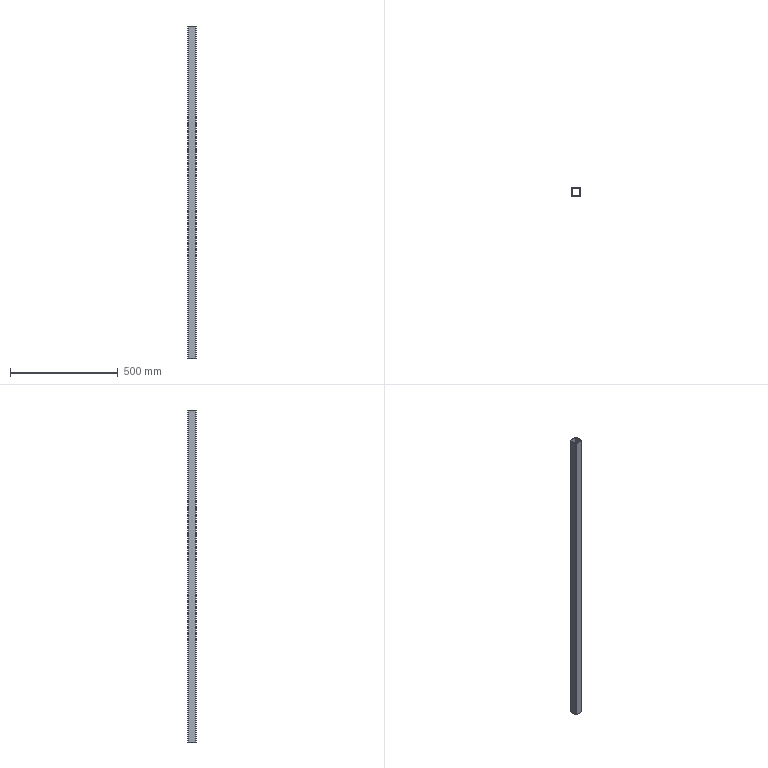Part | STEP file | X77-03115 | 1 solid | 14 faces | box 40 x 40 x 1540 mm | volume 671862 mm3 | plane 10 | cylinder 4 | commonest cylinder face diameters 6 x4
STEP:
#1=CARTESIAN_POINT('',(-20.,-17.,1540.));
#2=VERTEX_POINT('',#1);
#3=CARTESIAN_POINT('',(-17.,-20.,1540.));
#4=VERTEX_POINT('',#3);
#5=CARTESIAN_POINT('',(-17.,-17.,1540.));
#6=DIRECTION('',(0.,0.,1.));
#7=DIRECTION('',(-1.,0.,0.));
#8=AXIS2_PLACEMENT_3D('',#5,#6,#7);
#9=CIRCLE('',#8,3.);
#10=EDGE_CURVE('',#2,#4,#9,.T.);
#11=ORIENTED_EDGE('',*,*,#10,.T.);
#12=CARTESIAN_POINT('',(17.,-20.,1540.));
#13=VERTEX_POINT('',#12);
#14=CARTESIAN_POINT('',(-17.,-20.,1540.));
#15=DIRECTION('',(1.,0.,0.));
#16=VECTOR('',#15,1000.);
#17=LINE('',#14,#16);
#18=EDGE_CURVE('',#4,#13,#17,.T.);
#19=ORIENTED_EDGE('',*,*,#18,.T.);
#20=CARTESIAN_POINT('',(20.,-17.,1540.));
#21=VERTEX_POINT('',#20);
#22=CARTESIAN_POINT('',(17.,-17.,1540.));
#23=DIRECTION('',(0.,0.,1.));
#24=DIRECTION('',(-1.,0.,0.));
#25=AXIS2_PLACEMENT_3D('',#22,#23,#24);
#26=CIRCLE('',#25,3.);
#27=EDGE_CURVE('',#13,#21,#26,.T.);
#28=ORIENTED_EDGE('',*,*,#27,.T.);
#29=CARTESIAN_POINT('',(20.,17.,1540.));
#30=VERTEX_POINT('',#29);
#31=CARTESIAN_POINT('',(20.,-17.,1540.));
#32=DIRECTION('',(0.,1.,0.));
#33=VECTOR('',#32,1000.);
#34=LINE('',#31,#33);
#35=EDGE_CURVE('',#21,#30,#34,.T.);
#36=ORIENTED_EDGE('',*,*,#35,.T.);
#37=CARTESIAN_POINT('',(17.,20.,1540.));
#38=VERTEX_POINT('',#37);
#39=CARTESIAN_POINT('',(17.,17.,1540.));
#40=DIRECTION('',(0.,0.,1.));
#41=DIRECTION('',(1.,0.,0.));
#42=AXIS2_PLACEMENT_3D('',#39,#40,#41);
#43=CIRCLE('',#42,3.);
#44=EDGE_CURVE('',#30,#38,#43,.T.);
#45=ORIENTED_EDGE('',*,*,#44,.T.);
#46=CARTESIAN_POINT('',(-17.,20.,1540.));
#47=VERTEX_POINT('',#46);
#48=CARTESIAN_POINT('',(-17.,20.,1540.));
#49=DIRECTION('',(-1.,0.,0.));
#50=VECTOR('',#49,1000.);
#51=LINE('',#48,#50);
#52=EDGE_CURVE('',#38,#47,#51,.T.);
#53=ORIENTED_EDGE('',*,*,#52,.T.);
#54=CARTESIAN_POINT('',(-20.,17.,1540.));
#55=VERTEX_POINT('',#54);
#56=CARTESIAN_POINT('',(-17.,17.,1540.));
#57=DIRECTION('',(0.,0.,1.));
#58=DIRECTION('',(1.,0.,0.));
#59=AXIS2_PLACEMENT_3D('',#56,#57,#58);
#60=CIRCLE('',#59,3.);
#61=EDGE_CURVE('',#47,#55,#60,.T.);
#62=ORIENTED_EDGE('',*,*,#61,.T.);
#63=CARTESIAN_POINT('',(-20.,-17.,1540.));
#64=DIRECTION('',(0.,-1.,0.));
#65=VECTOR('',#64,1000.);
#66=LINE('',#63,#65);
#67=EDGE_CURVE('',#55,#2,#66,.T.);
#68=ORIENTED_EDGE('',*,*,#67,.T.);
#69=EDGE_LOOP('',(#11,#19,#28,#36,#45,#53,#62,#68));
#70=FACE_OUTER_BOUND('',#69,.T.);
#71=CARTESIAN_POINT('',(17.,-17.,1540.));
#72=VERTEX_POINT('',#71);
#73=CARTESIAN_POINT('',(17.,17.,1540.));
#74=VERTEX_POINT('',#73);
#75=CARTESIAN_POINT('',(17.,-17.,1540.));
#76=DIRECTION('',(0.,1.,0.));
#77=VECTOR('',#76,1000.);
#78=LINE('',#75,#77);
#79=EDGE_CURVE('',#72,#74,#78,.T.);
#80=ORIENTED_EDGE('',*,*,#79,.F.);
#81=CARTESIAN_POINT('',(-17.,-17.,1540.));
#82=VERTEX_POINT('',#81);
#83=CARTESIAN_POINT('',(-17.,-17.,1540.));
#84=DIRECTION('',(1.,0.,0.));
#85=VECTOR('',#84,1000.);
#86=LINE('',#83,#85);
#87=EDGE_CURVE('',#82,#72,#86,.T.);
#88=ORIENTED_EDGE('',*,*,#87,.F.);
#89=CARTESIAN_POINT('',(-17.,17.,1540.));
#90=VERTEX_POINT('',#89);
#91=CARTESIAN_POINT('',(-17.,-17.,1540.));
#92=DIRECTION('',(0.,-1.,0.));
#93=VECTOR('',#92,1000.);
#94=LINE('',#91,#93);
#95=EDGE_CURVE('',#90,#82,#94,.T.);
#96=ORIENTED_EDGE('',*,*,#95,.F.);
#97=CARTESIAN_POINT('',(-17.,17.,1540.));
#98=DIRECTION('',(-1.,0.,0.));
#99=VECTOR('',#98,1000.);
#100=LINE('',#97,#99);
#101=EDGE_CURVE('',#74,#90,#100,.T.);
#102=ORIENTED_EDGE('',*,*,#101,.F.);
#103=EDGE_LOOP('',(#80,#88,#96,#102));
#104=FACE_BOUND('',#103,.T.);
#105=CARTESIAN_POINT('',(-17.,-17.,1540.));
#106=DIRECTION('',(0.,0.,-1.));
#107=DIRECTION('',(-1.,0.,0.));
#108=AXIS2_PLACEMENT_3D('',#105,#106,#107);
#109=PLANE('',#108);
#110=ADVANCED_FACE('',(#70,#104),#109,.F.);
#111=CARTESIAN_POINT('',(-20.,-17.,0.));
#112=VERTEX_POINT('',#111);
#113=CARTESIAN_POINT('',(-17.,-20.,0.));
#114=VERTEX_POINT('',#113);
#115=CARTESIAN_POINT('',(-17.,-17.,0.));
#116=DIRECTION('',(0.,0.,1.));
#117=DIRECTION('',(-1.,0.,0.));
#118=AXIS2_PLACEMENT_3D('',#115,#116,#117);
#119=CIRCLE('',#118,3.);
#120=EDGE_CURVE('',#112,#114,#119,.T.);
#121=ORIENTED_EDGE('',*,*,#120,.F.);
#122=CARTESIAN_POINT('',(-20.,17.,0.));
#123=VERTEX_POINT('',#122);
#124=CARTESIAN_POINT('',(-20.,-17.,0.));
#125=DIRECTION('',(0.,-1.,0.));
#126=VECTOR('',#125,1000.);
#127=LINE('',#124,#126);
#128=EDGE_CURVE('',#123,#112,#127,.T.);
#129=ORIENTED_EDGE('',*,*,#128,.F.);
#130=CARTESIAN_POINT('',(-17.,20.,0.));
#131=VERTEX_POINT('',#130);
#132=CARTESIAN_POINT('',(-17.,17.,0.));
#133=DIRECTION('',(0.,0.,1.));
#134=DIRECTION('',(1.,0.,0.));
#135=AXIS2_PLACEMENT_3D('',#132,#133,#134);
#136=CIRCLE('',#135,3.);
#137=EDGE_CURVE('',#131,#123,#136,.T.);
#138=ORIENTED_EDGE('',*,*,#137,.F.);
#139=CARTESIAN_POINT('',(17.,20.,0.));
#140=VERTEX_POINT('',#139);
#141=CARTESIAN_POINT('',(-17.,20.,0.));
#142=DIRECTION('',(-1.,0.,0.));
#143=VECTOR('',#142,1000.);
#144=LINE('',#141,#143);
#145=EDGE_CURVE('',#140,#131,#144,.T.);
#146=ORIENTED_EDGE('',*,*,#145,.F.);
#147=CARTESIAN_POINT('',(20.,17.,0.));
#148=VERTEX_POINT('',#147);
#149=CARTESIAN_POINT('',(17.,17.,0.));
#150=DIRECTION('',(0.,0.,1.));
#151=DIRECTION('',(1.,0.,0.));
#152=AXIS2_PLACEMENT_3D('',#149,#150,#151);
#153=CIRCLE('',#152,3.);
#154=EDGE_CURVE('',#148,#140,#153,.T.);
#155=ORIENTED_EDGE('',*,*,#154,.F.);
#156=CARTESIAN_POINT('',(20.,-17.,0.));
#157=VERTEX_POINT('',#156);
#158=CARTESIAN_POINT('',(20.,-17.,0.));
#159=DIRECTION('',(0.,1.,0.));
#160=VECTOR('',#159,1000.);
#161=LINE('',#158,#160);
#162=EDGE_CURVE('',#157,#148,#161,.T.);
#163=ORIENTED_EDGE('',*,*,#162,.F.);
#164=CARTESIAN_POINT('',(17.,-20.,0.));
#165=VERTEX_POINT('',#164);
#166=CARTESIAN_POINT('',(17.,-17.,0.));
#167=DIRECTION('',(0.,0.,1.));
#168=DIRECTION('',(-1.,0.,0.));
#169=AXIS2_PLACEMENT_3D('',#166,#167,#168);
#170=CIRCLE('',#169,3.);
#171=EDGE_CURVE('',#165,#157,#170,.T.);
#172=ORIENTED_EDGE('',*,*,#171,.F.);
#173=CARTESIAN_POINT('',(-17.,-20.,0.));
#174=DIRECTION('',(1.,0.,0.));
#175=VECTOR('',#174,1000.);
#176=LINE('',#173,#175);
#177=EDGE_CURVE('',#114,#165,#176,.T.);
#178=ORIENTED_EDGE('',*,*,#177,.F.);
#179=EDGE_LOOP('',(#121,#129,#138,#146,#155,#163,#172,#178));
#180=FACE_OUTER_BOUND('',#179,.T.);
#181=CARTESIAN_POINT('',(-17.,-17.,0.));
#182=VERTEX_POINT('',#181);
#183=CARTESIAN_POINT('',(17.,-17.,0.));
#184=VERTEX_POINT('',#183);
#185=CARTESIAN_POINT('',(-17.,-17.,0.));
#186=DIRECTION('',(1.,0.,0.));
#187=VECTOR('',#186,1000.);
#188=LINE('',#185,#187);
#189=EDGE_CURVE('',#182,#184,#188,.T.);
#190=ORIENTED_EDGE('',*,*,#189,.T.);
#191=CARTESIAN_POINT('',(17.,17.,0.));
#192=VERTEX_POINT('',#191);
#193=CARTESIAN_POINT('',(17.,-17.,0.));
#194=DIRECTION('',(0.,1.,0.));
#195=VECTOR('',#194,1000.);
#196=LINE('',#193,#195);
#197=EDGE_CURVE('',#184,#192,#196,.T.);
#198=ORIENTED_EDGE('',*,*,#197,.T.);
#199=CARTESIAN_POINT('',(-17.,17.,0.));
#200=VERTEX_POINT('',#199);
#201=CARTESIAN_POINT('',(-17.,17.,0.));
#202=DIRECTION('',(-1.,0.,0.));
#203=VECTOR('',#202,1000.);
#204=LINE('',#201,#203);
#205=EDGE_CURVE('',#192,#200,#204,.T.);
#206=ORIENTED_EDGE('',*,*,#205,.T.);
#207=CARTESIAN_POINT('',(-17.,-17.,0.));
#208=DIRECTION('',(0.,-1.,0.));
#209=VECTOR('',#208,1000.);
#210=LINE('',#207,#209);
#211=EDGE_CURVE('',#200,#182,#210,.T.);
#212=ORIENTED_EDGE('',*,*,#211,.T.);
#213=EDGE_LOOP('',(#190,#198,#206,#212));
#214=FACE_BOUND('',#213,.T.);
#215=CARTESIAN_POINT('',(-17.,-17.,0.));
#216=DIRECTION('',(0.,0.,-1.));
#217=DIRECTION('',(-1.,0.,0.));
#218=AXIS2_PLACEMENT_3D('',#215,#216,#217);
#219=PLANE('',#218);
#220=ADVANCED_FACE('',(#180,#214),#219,.T.);
#221=ORIENTED_EDGE('',*,*,#120,.T.);
#222=CARTESIAN_POINT('',(-17.,-20.,1540.));
#223=DIRECTION('',(0.,0.,-1.));
#224=VECTOR('',#223,1000.);
#225=LINE('',#222,#224);
#226=EDGE_CURVE('',#4,#114,#225,.T.);
#227=ORIENTED_EDGE('',*,*,#226,.F.);
#228=ORIENTED_EDGE('',*,*,#10,.F.);
#229=CARTESIAN_POINT('',(-20.,-17.,1540.));
#230=DIRECTION('',(0.,0.,-1.));
#231=VECTOR('',#230,1000.);
#232=LINE('',#229,#231);
#233=EDGE_CURVE('',#2,#112,#232,.T.);
#234=ORIENTED_EDGE('',*,*,#233,.T.);
#235=EDGE_LOOP('',(#221,#227,#228,#234));
#236=FACE_OUTER_BOUND('',#235,.T.);
#237=CARTESIAN_POINT('',(-17.,-17.,1540.));
#238=DIRECTION('',(0.,0.,-1.));
#239=DIRECTION('',(-1.,0.,0.));
#240=AXIS2_PLACEMENT_3D('',#237,#238,#239);
#241=CYLINDRICAL_SURFACE('',#240,3.);
#242=ADVANCED_FACE('',(#236),#241,.T.);
#243=ORIENTED_EDGE('',*,*,#177,.T.);
#244=CARTESIAN_POINT('',(17.,-20.,1540.));
#245=DIRECTION('',(0.,0.,-1.));
#246=VECTOR('',#245,1000.);
#247=LINE('',#244,#246);
#248=EDGE_CURVE('',#13,#165,#247,.T.);
#249=ORIENTED_EDGE('',*,*,#248,.F.);
#250=ORIENTED_EDGE('',*,*,#18,.F.);
#251=ORIENTED_EDGE('',*,*,#226,.T.);
#252=EDGE_LOOP('',(#243,#249,#250,#251));
#253=FACE_OUTER_BOUND('',#252,.T.);
#254=CARTESIAN_POINT('',(-17.,-20.,1540.));
#255=DIRECTION('',(0.,1.,0.));
#256=DIRECTION('',(0.,0.,1.));
#257=AXIS2_PLACEMENT_3D('',#254,#255,#256);
#258=PLANE('',#257);
#259=ADVANCED_FACE('',(#253),#258,.F.);
#260=ORIENTED_EDGE('',*,*,#171,.T.);
#261=CARTESIAN_POINT('',(20.,-17.,1540.));
#262=DIRECTION('',(0.,0.,-1.));
#263=VECTOR('',#262,1000.);
#264=LINE('',#261,#263);
#265=EDGE_CURVE('',#21,#157,#264,.T.);
#266=ORIENTED_EDGE('',*,*,#265,.F.);
#267=ORIENTED_EDGE('',*,*,#27,.F.);
#268=ORIENTED_EDGE('',*,*,#248,.T.);
#269=EDGE_LOOP('',(#260,#266,#267,#268));
#270=FACE_OUTER_BOUND('',#269,.T.);
#271=CARTESIAN_POINT('',(17.,-17.,1540.));
#272=DIRECTION('',(0.,0.,-1.));
#273=DIRECTION('',(-1.,0.,0.));
#274=AXIS2_PLACEMENT_3D('',#271,#272,#273);
#275=CYLINDRICAL_SURFACE('',#274,3.);
#276=ADVANCED_FACE('',(#270),#275,.T.);
#277=ORIENTED_EDGE('',*,*,#162,.T.);
#278=CARTESIAN_POINT('',(20.,17.,1540.));
#279=DIRECTION('',(0.,0.,-1.));
#280=VECTOR('',#279,1000.);
#281=LINE('',#278,#280);
#282=EDGE_CURVE('',#30,#148,#281,.T.);
#283=ORIENTED_EDGE('',*,*,#282,.F.);
#284=ORIENTED_EDGE('',*,*,#35,.F.);
#285=ORIENTED_EDGE('',*,*,#265,.T.);
#286=EDGE_LOOP('',(#277,#283,#284,#285));
#287=FACE_OUTER_BOUND('',#286,.T.);
#288=CARTESIAN_POINT('',(20.,-17.,1540.));
#289=DIRECTION('',(-1.,0.,0.));
#290=DIRECTION('',(0.,0.,1.));
#291=AXIS2_PLACEMENT_3D('',#288,#289,#290);
#292=PLANE('',#291);
#293=ADVANCED_FACE('',(#287),#292,.F.);
#294=ORIENTED_EDGE('',*,*,#154,.T.);
#295=CARTESIAN_POINT('',(17.,20.,1540.));
#296=DIRECTION('',(0.,0.,-1.));
#297=VECTOR('',#296,1000.);
#298=LINE('',#295,#297);
#299=EDGE_CURVE('',#38,#140,#298,.T.);
#300=ORIENTED_EDGE('',*,*,#299,.F.);
#301=ORIENTED_EDGE('',*,*,#44,.F.);
#302=ORIENTED_EDGE('',*,*,#282,.T.);
#303=EDGE_LOOP('',(#294,#300,#301,#302));
#304=FACE_OUTER_BOUND('',#303,.T.);
#305=CARTESIAN_POINT('',(17.,17.,1540.));
#306=DIRECTION('',(0.,0.,-1.));
#307=DIRECTION('',(-1.,0.,0.));
#308=AXIS2_PLACEMENT_3D('',#305,#306,#307);
#309=CYLINDRICAL_SURFACE('',#308,3.);
#310=ADVANCED_FACE('',(#304),#309,.T.);
#311=ORIENTED_EDGE('',*,*,#145,.T.);
#312=CARTESIAN_POINT('',(-17.,20.,1540.));
#313=DIRECTION('',(0.,0.,-1.));
#314=VECTOR('',#313,1000.);
#315=LINE('',#312,#314);
#316=EDGE_CURVE('',#47,#131,#315,.T.);
#317=ORIENTED_EDGE('',*,*,#316,.F.);
#318=ORIENTED_EDGE('',*,*,#52,.F.);
#319=ORIENTED_EDGE('',*,*,#299,.T.);
#320=EDGE_LOOP('',(#311,#317,#318,#319));
#321=FACE_OUTER_BOUND('',#320,.T.);
#322=CARTESIAN_POINT('',(-17.,20.,1540.));
#323=DIRECTION('',(0.,-1.,0.));
#324=DIRECTION('',(0.,0.,-1.));
#325=AXIS2_PLACEMENT_3D('',#322,#323,#324);
#326=PLANE('',#325);
#327=ADVANCED_FACE('',(#321),#326,.F.);
#328=ORIENTED_EDGE('',*,*,#137,.T.);
#329=CARTESIAN_POINT('',(-20.,17.,1540.));
#330=DIRECTION('',(0.,0.,-1.));
#331=VECTOR('',#330,1000.);
#332=LINE('',#329,#331);
#333=EDGE_CURVE('',#55,#123,#332,.T.);
#334=ORIENTED_EDGE('',*,*,#333,.F.);
#335=ORIENTED_EDGE('',*,*,#61,.F.);
#336=ORIENTED_EDGE('',*,*,#316,.T.);
#337=EDGE_LOOP('',(#328,#334,#335,#336));
#338=FACE_OUTER_BOUND('',#337,.T.);
#339=CARTESIAN_POINT('',(-17.,17.,1540.));
#340=DIRECTION('',(0.,0.,-1.));
#341=DIRECTION('',(-1.,0.,0.));
#342=AXIS2_PLACEMENT_3D('',#339,#340,#341);
#343=CYLINDRICAL_SURFACE('',#342,3.);
#344=ADVANCED_FACE('',(#338),#343,.T.);
#345=ORIENTED_EDGE('',*,*,#128,.T.);
#346=ORIENTED_EDGE('',*,*,#233,.F.);
#347=ORIENTED_EDGE('',*,*,#67,.F.);
#348=ORIENTED_EDGE('',*,*,#333,.T.);
#349=EDGE_LOOP('',(#345,#346,#347,#348));
#350=FACE_OUTER_BOUND('',#349,.T.);
#351=CARTESIAN_POINT('',(-20.,-17.,1540.));
#352=DIRECTION('',(1.,0.,0.));
#353=DIRECTION('',(0.,0.,-1.));
#354=AXIS2_PLACEMENT_3D('',#351,#352,#353);
#355=PLANE('',#354);
#356=ADVANCED_FACE('',(#350),#355,.F.);
#357=ORIENTED_EDGE('',*,*,#197,.F.);
#358=CARTESIAN_POINT('',(17.,-17.,1540.));
#359=DIRECTION('',(0.,0.,-1.));
#360=VECTOR('',#359,1000.);
#361=LINE('',#358,#360);
#362=EDGE_CURVE('',#72,#184,#361,.T.);
#363=ORIENTED_EDGE('',*,*,#362,.F.);
#364=ORIENTED_EDGE('',*,*,#79,.T.);
#365=CARTESIAN_POINT('',(17.,17.,1540.));
#366=DIRECTION('',(0.,0.,-1.));
#367=VECTOR('',#366,1000.);
#368=LINE('',#365,#367);
#369=EDGE_CURVE('',#74,#192,#368,.T.);
#370=ORIENTED_EDGE('',*,*,#369,.T.);
#371=EDGE_LOOP('',(#357,#363,#364,#370));
#372=FACE_OUTER_BOUND('',#371,.T.);
#373=CARTESIAN_POINT('',(17.,-17.,1540.));
#374=DIRECTION('',(-1.,0.,0.));
#375=DIRECTION('',(0.,0.,1.));
#376=AXIS2_PLACEMENT_3D('',#373,#374,#375);
#377=PLANE('',#376);
#378=ADVANCED_FACE('',(#372),#377,.T.);
#379=ORIENTED_EDGE('',*,*,#205,.F.);
#380=ORIENTED_EDGE('',*,*,#369,.F.);
#381=ORIENTED_EDGE('',*,*,#101,.T.);
#382=CARTESIAN_POINT('',(-17.,17.,1540.));
#383=DIRECTION('',(0.,0.,-1.));
#384=VECTOR('',#383,1000.);
#385=LINE('',#382,#384);
#386=EDGE_CURVE('',#90,#200,#385,.T.);
#387=ORIENTED_EDGE('',*,*,#386,.T.);
#388=EDGE_LOOP('',(#379,#380,#381,#387));
#389=FACE_OUTER_BOUND('',#388,.T.);
#390=CARTESIAN_POINT('',(-17.,17.,1540.));
#391=DIRECTION('',(0.,-1.,0.));
#392=DIRECTION('',(0.,0.,-1.));
#393=AXIS2_PLACEMENT_3D('',#390,#391,#392);
#394=PLANE('',#393);
#395=ADVANCED_FACE('',(#389),#394,.T.);
#396=ORIENTED_EDGE('',*,*,#211,.F.);
#397=ORIENTED_EDGE('',*,*,#386,.F.);
#398=ORIENTED_EDGE('',*,*,#95,.T.);
#399=CARTESIAN_POINT('',(-17.,-17.,1540.));
#400=DIRECTION('',(0.,0.,-1.));
#401=VECTOR('',#400,1000.);
#402=LINE('',#399,#401);
#403=EDGE_CURVE('',#82,#182,#402,.T.);
#404=ORIENTED_EDGE('',*,*,#403,.T.);
#405=EDGE_LOOP('',(#396,#397,#398,#404));
#406=FACE_OUTER_BOUND('',#405,.T.);
#407=CARTESIAN_POINT('',(-17.,-17.,1540.));
#408=DIRECTION('',(1.,0.,0.));
#409=DIRECTION('',(0.,0.,-1.));
#410=AXIS2_PLACEMENT_3D('',#407,#408,#409);
#411=PLANE('',#410);
#412=ADVANCED_FACE('',(#406),#411,.T.);
#413=ORIENTED_EDGE('',*,*,#189,.F.);
#414=ORIENTED_EDGE('',*,*,#403,.F.);
#415=ORIENTED_EDGE('',*,*,#87,.T.);
#416=ORIENTED_EDGE('',*,*,#362,.T.);
#417=EDGE_LOOP('',(#413,#414,#415,#416));
#418=FACE_OUTER_BOUND('',#417,.T.);
#419=CARTESIAN_POINT('',(-17.,-17.,1540.));
#420=DIRECTION('',(0.,1.,0.));
#421=DIRECTION('',(0.,0.,1.));
#422=AXIS2_PLACEMENT_3D('',#419,#420,#421);
#423=PLANE('',#422);
#424=ADVANCED_FACE('',(#418),#423,.T.);
#425=CLOSED_SHELL('',(#110,#220,#242,#259,#276,#293,#310,#327,#344,#356,#378,#395,#412,#424));
#426=MANIFOLD_SOLID_BREP('',#425);
#427=CARTESIAN_POINT('',(0.,0.,0.));
#428=DIRECTION('',(0.,0.,1.));
#429=DIRECTION('',(1.,0.,0.));
#430=AXIS2_PLACEMENT_3D('',#427,#428,#429);
#431=(LENGTH_UNIT()NAMED_UNIT(*)SI_UNIT(.MILLI.,.METRE.));
#432=UNCERTAINTY_MEASURE_WITH_UNIT(LENGTH_MEASURE(0.00001),#431,'','');
#433=(NAMED_UNIT(*)PLANE_ANGLE_UNIT()SI_UNIT($,.RADIAN.));
#434=(NAMED_UNIT(*)SI_UNIT($,.STERADIAN.)SOLID_ANGLE_UNIT());
#435=(GEOMETRIC_REPRESENTATION_CONTEXT(3)GLOBAL_UNCERTAINTY_ASSIGNED_CONTEXT((#432))GLOBAL_UNIT_ASSIGNED_CONTEXT((#431,#433,#434))REPRESENTATION_CONTEXT('',''));
#436=ADVANCED_BREP_SHAPE_REPRESENTATION('',(#426,#430),#435);